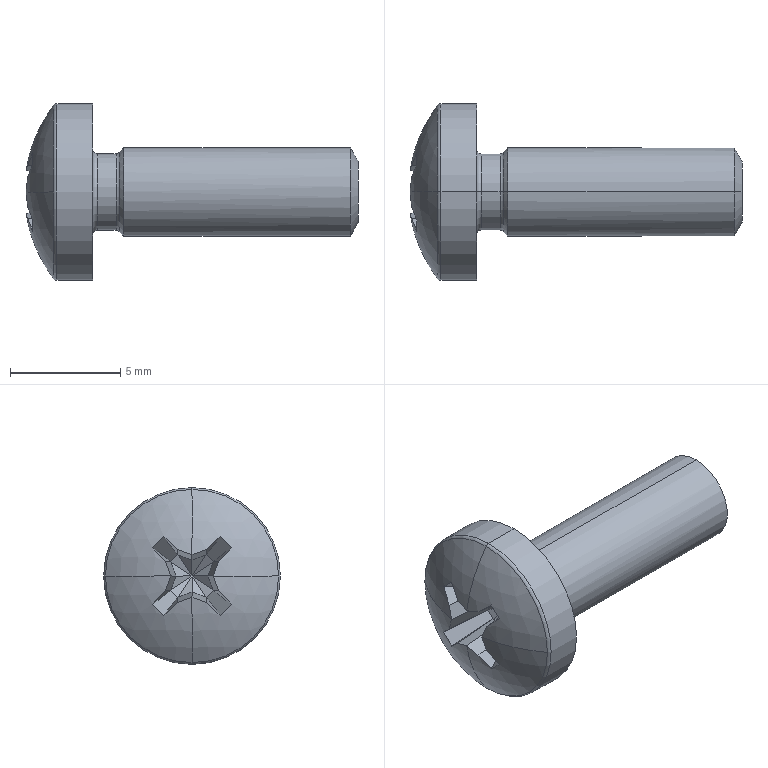Part | STEP file | 103000010384_M4×12 | 1 solid | 54 faces | box 15.027 x 8 x 8 mm | volume 256.338 mm3 | plane 34 | cylinder 6 | torus 6 | cone 4 | sphere 4 | commonest cylinder face diameters 3.464 x2 4 x2 8 x2
STEP:
#1=CARTESIAN_POINT('',(15.1,0.,1.394));
#2=VERTEX_POINT('',#1);
#3=CARTESIAN_POINT('',(15.1,0.,-1.394));
#4=VERTEX_POINT('',#3);
#5=CARTESIAN_POINT('',(15.1,0.,0.));
#6=DIRECTION('',(-1.,0.,0.));
#7=AXIS2_PLACEMENT_3D('',#5,#6,$);
#8=CIRCLE('',#7,1.394);
#9=EDGE_CURVE('',#2,#4,#8,.T.);
#10=ORIENTED_EDGE('',*,*,#9,.T.);
#11=CARTESIAN_POINT('',(14.754,0.,-2.));
#12=VERTEX_POINT('',#11);
#13=CARTESIAN_POINT('',(-247950.901,0.,-434181.551));
#14=DIRECTION('',(-0.4959,0.,-0.8684));
#15=VECTOR('',#14,1.);
#16=LINE('',#13,#15);
#17=EDGE_CURVE('',#4,#12,#16,.T.);
#18=ORIENTED_EDGE('',*,*,#17,.T.);
#19=CARTESIAN_POINT('',(14.754,0.,2.));
#20=VERTEX_POINT('',#19);
#21=CARTESIAN_POINT('',(14.754,0.,0.));
#22=DIRECTION('',(-1.,0.,0.));
#23=AXIS2_PLACEMENT_3D('',#21,#22,$);
#24=CIRCLE('',#23,2.);
#25=EDGE_CURVE('',#20,#12,#24,.T.);
#26=ORIENTED_EDGE('',*,*,#25,.F.);
#27=CARTESIAN_POINT('',(-247950.901,0.,434181.551));
#28=DIRECTION('',(-0.4959,0.,0.8684));
#29=VECTOR('',#28,1.);
#30=LINE('',#27,#29);
#31=EDGE_CURVE('',#2,#20,#30,.T.);
#32=ORIENTED_EDGE('',*,*,#31,.F.);
#33=EDGE_LOOP('',(#10,#18,#26,#32));
#34=FACE_OUTER_BOUND('',#33,.T.);
#35=CARTESIAN_POINT('',(14.754,0.,0.));
#36=DIRECTION('',(-1.,0.,0.));
#37=DIRECTION('',(0.,0.,1.));
#38=AXIS2_PLACEMENT_3D('',#35,#36,#37);
#39=CONICAL_SURFACE('',#38,2.,1.052);
#40=ADVANCED_FACE('',(#34),#39,.T.);
#41=ORIENTED_EDGE('',*,*,#9,.F.);
#42=CARTESIAN_POINT('',(15.1,0.,0.));
#43=DIRECTION('',(-1.,0.,0.));
#44=AXIS2_PLACEMENT_3D('',#42,#43,$);
#45=CIRCLE('',#44,1.394);
#46=EDGE_CURVE('',#4,#2,#45,.T.);
#47=ORIENTED_EDGE('',*,*,#46,.F.);
#48=EDGE_LOOP('',(#41,#47));
#49=FACE_OUTER_BOUND('',#48,.T.);
#50=CARTESIAN_POINT('',(15.1,0.,0.));
#51=DIRECTION('',(-1.,0.,0.));
#52=DIRECTION('',(0.,0.,1.));
#53=AXIS2_PLACEMENT_3D('',#50,#51,#52);
#54=PLANE('',#53);
#55=ADVANCED_FACE('',(#49),#54,.F.);
#56=ORIENTED_EDGE('',*,*,#17,.F.);
#57=ORIENTED_EDGE('',*,*,#46,.T.);
#58=ORIENTED_EDGE('',*,*,#31,.T.);
#59=CARTESIAN_POINT('',(14.754,0.,0.));
#60=DIRECTION('',(-1.,0.,0.));
#61=AXIS2_PLACEMENT_3D('',#59,#60,$);
#62=CIRCLE('',#61,2.);
#63=EDGE_CURVE('',#12,#20,#62,.T.);
#64=ORIENTED_EDGE('',*,*,#63,.F.);
#65=EDGE_LOOP('',(#56,#57,#58,#64));
#66=FACE_OUTER_BOUND('',#65,.T.);
#67=CARTESIAN_POINT('',(14.754,0.,0.));
#68=DIRECTION('',(-1.,0.,0.));
#69=DIRECTION('',(0.,0.,-1.));
#70=AXIS2_PLACEMENT_3D('',#67,#68,#69);
#71=CONICAL_SURFACE('',#70,2.,1.052);
#72=ADVANCED_FACE('',(#66),#71,.T.);
#73=ORIENTED_EDGE('',*,*,#25,.T.);
#74=CARTESIAN_POINT('',(4.5,0.,-2.));
#75=VERTEX_POINT('',#74);
#76=CARTESIAN_POINT('',(-3.442,0.,-2.));
#77=DIRECTION('',(-1.,0.,0.));
#78=VECTOR('',#77,1.);
#79=LINE('',#76,#78);
#80=EDGE_CURVE('',#12,#75,#79,.T.);
#81=ORIENTED_EDGE('',*,*,#80,.T.);
#82=CARTESIAN_POINT('',(4.5,0.,2.));
#83=VERTEX_POINT('',#82);
#84=CARTESIAN_POINT('',(4.5,0.,2.));
#85=CARTESIAN_POINT('',(4.5,0.6283,2.));
#86=CARTESIAN_POINT('',(4.5,1.257,1.753));
#87=CARTESIAN_POINT('',(4.5,1.753,1.257));
#88=CARTESIAN_POINT('',(4.5,2.247,0.));
#89=CARTESIAN_POINT('',(4.5,1.753,-1.257));
#90=CARTESIAN_POINT('',(4.5,1.257,-1.753));
#91=CARTESIAN_POINT('',(4.5,0.6283,-2.));
#92=CARTESIAN_POINT('',(4.5,0.,-2.));
#93=B_SPLINE_CURVE_WITH_KNOTS('',5,(#84,#85,#86,#87,#88,#89,#90,#91,#92),.UNSPECIFIED.,.F.,.U.,(6,3,6),(-3.142,0.,3.142),.UNSPECIFIED.);
#94=EDGE_CURVE('',#83,#75,#93,.T.);
#95=ORIENTED_EDGE('',*,*,#94,.F.);
#96=CARTESIAN_POINT('',(-3.442,0.,2.));
#97=DIRECTION('',(-1.,0.,0.));
#98=VECTOR('',#97,1.);
#99=LINE('',#96,#98);
#100=EDGE_CURVE('',#20,#83,#99,.T.);
#101=ORIENTED_EDGE('',*,*,#100,.F.);
#102=EDGE_LOOP('',(#73,#81,#95,#101));
#103=FACE_OUTER_BOUND('',#102,.T.);
#104=CARTESIAN_POINT('',(-3.442,0.,0.));
#105=DIRECTION('',(-1.,0.,0.));
#106=DIRECTION('',(0.,0.,1.));
#107=AXIS2_PLACEMENT_3D('',#104,#105,#106);
#108=CYLINDRICAL_SURFACE('',#107,2.);
#109=ADVANCED_FACE('',(#103),#108,.T.);
#110=ORIENTED_EDGE('',*,*,#80,.F.);
#111=ORIENTED_EDGE('',*,*,#63,.T.);
#112=ORIENTED_EDGE('',*,*,#100,.T.);
#113=CARTESIAN_POINT('',(4.5,0.,-2.));
#114=CARTESIAN_POINT('',(4.5,-0.6283,-2.));
#115=CARTESIAN_POINT('',(4.5,-1.257,-1.753));
#116=CARTESIAN_POINT('',(4.5,-1.753,-1.257));
#117=CARTESIAN_POINT('',(4.5,-2.247,0.));
#118=CARTESIAN_POINT('',(4.5,-1.753,1.257));
#119=CARTESIAN_POINT('',(4.5,-1.257,1.753));
#120=CARTESIAN_POINT('',(4.5,-0.6283,2.));
#121=CARTESIAN_POINT('',(4.5,0.,2.));
#122=B_SPLINE_CURVE_WITH_KNOTS('',5,(#113,#114,#115,#116,#117,#118,#119,#120,#121),.UNSPECIFIED.,.F.,.U.,(6,3,6),(-3.142,0.,3.142),.UNSPECIFIED.);
#123=EDGE_CURVE('',#75,#83,#122,.T.);
#124=ORIENTED_EDGE('',*,*,#123,.F.);
#125=EDGE_LOOP('',(#110,#111,#112,#124));
#126=FACE_OUTER_BOUND('',#125,.T.);
#127=CARTESIAN_POINT('',(-3.442,0.,0.));
#128=DIRECTION('',(-1.,0.,0.));
#129=DIRECTION('',(0.,0.,-1.));
#130=AXIS2_PLACEMENT_3D('',#127,#128,#129);
#131=CYLINDRICAL_SURFACE('',#130,2.);
#132=ADVANCED_FACE('',(#126),#131,.T.);
#133=CARTESIAN_POINT('',(4.291,0.,-1.791));
#134=VERTEX_POINT('',#133);
#135=CARTESIAN_POINT('',(4.291,0.,1.791));
#136=VERTEX_POINT('',#135);
#137=CARTESIAN_POINT('',(4.291,0.,0.));
#138=DIRECTION('',(1.,0.,0.));
#139=AXIS2_PLACEMENT_3D('',#137,#138,$);
#140=CIRCLE('',#139,1.791);
#141=EDGE_CURVE('',#134,#136,#140,.T.);
#142=ORIENTED_EDGE('',*,*,#141,.T.);
#143=CARTESIAN_POINT('',(353556.891,0.,353554.391));
#144=DIRECTION('',(0.7071,0.,0.7071));
#145=VECTOR('',#144,1.);
#146=LINE('',#143,#145);
#147=EDGE_CURVE('',#136,#83,#146,.T.);
#148=ORIENTED_EDGE('',*,*,#147,.T.);
#149=ORIENTED_EDGE('',*,*,#94,.T.);
#150=CARTESIAN_POINT('',(353556.891,0.,-353554.391));
#151=DIRECTION('',(0.7071,0.,-0.7071));
#152=VECTOR('',#151,1.);
#153=LINE('',#150,#152);
#154=EDGE_CURVE('',#134,#75,#153,.T.);
#155=ORIENTED_EDGE('',*,*,#154,.F.);
#156=EDGE_LOOP('',(#142,#148,#149,#155));
#157=FACE_OUTER_BOUND('',#156,.T.);
#158=CARTESIAN_POINT('',(4.5,0.,0.));
#159=DIRECTION('',(1.,0.,0.));
#160=DIRECTION('',(0.,0.,-1.));
#161=AXIS2_PLACEMENT_3D('',#158,#159,#160);
#162=CONICAL_SURFACE('',#161,2.,0.7854);
#163=ADVANCED_FACE('',(#157),#162,.T.);
#164=ORIENTED_EDGE('',*,*,#147,.F.);
#165=CARTESIAN_POINT('',(4.291,0.,0.));
#166=DIRECTION('',(1.,0.,0.));
#167=AXIS2_PLACEMENT_3D('',#165,#166,$);
#168=CIRCLE('',#167,1.791);
#169=EDGE_CURVE('',#136,#134,#168,.T.);
#170=ORIENTED_EDGE('',*,*,#169,.T.);
#171=ORIENTED_EDGE('',*,*,#154,.T.);
#172=ORIENTED_EDGE('',*,*,#123,.T.);
#173=EDGE_LOOP('',(#164,#170,#171,#172));
#174=FACE_OUTER_BOUND('',#173,.T.);
#175=CARTESIAN_POINT('',(4.5,0.,0.));
#176=DIRECTION('',(1.,0.,0.));
#177=DIRECTION('',(0.,0.,1.));
#178=AXIS2_PLACEMENT_3D('',#175,#176,#177);
#179=CONICAL_SURFACE('',#178,2.,0.7854);
#180=ADVANCED_FACE('',(#174),#179,.T.);
#181=CARTESIAN_POINT('',(4.149,0.,-1.732));
#182=VERTEX_POINT('',#181);
#183=CARTESIAN_POINT('',(4.149,0.,-1.932));
#184=DIRECTION('',(0.,1.,0.));
#185=AXIS2_PLACEMENT_3D('',#183,#184,$);
#186=CIRCLE('',#185,0.2);
#187=EDGE_CURVE('',#182,#134,#186,.T.);
#188=ORIENTED_EDGE('',*,*,#187,.F.);
#189=CARTESIAN_POINT('',(4.149,0.,1.732));
#190=VERTEX_POINT('',#189);
#191=CARTESIAN_POINT('',(4.149,0.,0.));
#192=DIRECTION('',(-1.,0.,0.));
#193=AXIS2_PLACEMENT_3D('',#191,#192,$);
#194=CIRCLE('',#193,1.732);
#195=EDGE_CURVE('',#190,#182,#194,.T.);
#196=ORIENTED_EDGE('',*,*,#195,.F.);
#197=CARTESIAN_POINT('',(4.149,0.,1.932));
#198=DIRECTION('',(0.,-1.,0.));
#199=AXIS2_PLACEMENT_3D('',#197,#198,$);
#200=CIRCLE('',#199,0.2);
#201=EDGE_CURVE('',#190,#136,#200,.T.);
#202=ORIENTED_EDGE('',*,*,#201,.T.);
#203=ORIENTED_EDGE('',*,*,#141,.F.);
#204=EDGE_LOOP('',(#188,#196,#202,#203));
#205=FACE_OUTER_BOUND('',#204,.T.);
#206=CARTESIAN_POINT('',(4.149,0.,0.));
#207=DIRECTION('',(-1.,0.,0.));
#208=DIRECTION('',(0.,0.,1.));
#209=AXIS2_PLACEMENT_3D('',#206,#207,#208);
#210=TOROIDAL_SURFACE('',#209,1.932,0.2);
#211=ADVANCED_FACE('',(#205),#210,.F.);
#212=CARTESIAN_POINT('',(4.149,0.,0.));
#213=DIRECTION('',(-1.,0.,0.));
#214=AXIS2_PLACEMENT_3D('',#212,#213,$);
#215=CIRCLE('',#214,1.732);
#216=EDGE_CURVE('',#182,#190,#215,.T.);
#217=ORIENTED_EDGE('',*,*,#216,.F.);
#218=ORIENTED_EDGE('',*,*,#187,.T.);
#219=ORIENTED_EDGE('',*,*,#169,.F.);
#220=ORIENTED_EDGE('',*,*,#201,.F.);
#221=EDGE_LOOP('',(#217,#218,#219,#220));
#222=FACE_OUTER_BOUND('',#221,.T.);
#223=CARTESIAN_POINT('',(4.149,0.,0.));
#224=DIRECTION('',(-1.,0.,0.));
#225=DIRECTION('',(0.,0.,-1.));
#226=AXIS2_PLACEMENT_3D('',#223,#224,#225);
#227=TOROIDAL_SURFACE('',#226,1.932,0.2);
#228=ADVANCED_FACE('',(#222),#227,.F.);
#229=ORIENTED_EDGE('',*,*,#195,.T.);
#230=CARTESIAN_POINT('',(3.3,0.,-1.732));
#231=VERTEX_POINT('',#230);
#232=CARTESIAN_POINT('',(-3.442,0.,-1.732));
#233=DIRECTION('',(-1.,0.,0.));
#234=VECTOR('',#233,1.);
#235=LINE('',#232,#234);
#236=EDGE_CURVE('',#182,#231,#235,.T.);
#237=ORIENTED_EDGE('',*,*,#236,.T.);
#238=CARTESIAN_POINT('',(3.3,0.,1.732));
#239=VERTEX_POINT('',#238);
#240=CARTESIAN_POINT('',(3.3,0.,0.));
#241=DIRECTION('',(-1.,0.,0.));
#242=AXIS2_PLACEMENT_3D('',#240,#241,$);
#243=CIRCLE('',#242,1.732);
#244=EDGE_CURVE('',#231,#239,#243,.F.);
#245=ORIENTED_EDGE('',*,*,#244,.T.);
#246=CARTESIAN_POINT('',(-3.442,0.,1.732));
#247=DIRECTION('',(-1.,0.,0.));
#248=VECTOR('',#247,1.);
#249=LINE('',#246,#248);
#250=EDGE_CURVE('',#190,#239,#249,.T.);
#251=ORIENTED_EDGE('',*,*,#250,.F.);
#252=EDGE_LOOP('',(#229,#237,#245,#251));
#253=FACE_OUTER_BOUND('',#252,.T.);
#254=CARTESIAN_POINT('',(-3.442,0.,0.));
#255=DIRECTION('',(-1.,0.,0.));
#256=DIRECTION('',(0.,0.,1.));
#257=AXIS2_PLACEMENT_3D('',#254,#255,#256);
#258=CYLINDRICAL_SURFACE('',#257,1.732);
#259=ADVANCED_FACE('',(#253),#258,.T.);
#260=ORIENTED_EDGE('',*,*,#236,.F.);
#261=ORIENTED_EDGE('',*,*,#216,.T.);
#262=ORIENTED_EDGE('',*,*,#250,.T.);
#263=CARTESIAN_POINT('',(3.3,0.,0.));
#264=DIRECTION('',(-1.,0.,0.));
#265=AXIS2_PLACEMENT_3D('',#263,#264,$);
#266=CIRCLE('',#265,1.732);
#267=EDGE_CURVE('',#239,#231,#266,.F.);
#268=ORIENTED_EDGE('',*,*,#267,.T.);
#269=EDGE_LOOP('',(#260,#261,#262,#268));
#270=FACE_OUTER_BOUND('',#269,.T.);
#271=CARTESIAN_POINT('',(-3.442,0.,0.));
#272=DIRECTION('',(-1.,0.,0.));
#273=DIRECTION('',(0.,0.,-1.));
#274=AXIS2_PLACEMENT_3D('',#271,#272,#273);
#275=CYLINDRICAL_SURFACE('',#274,1.732);
#276=ADVANCED_FACE('',(#270),#275,.T.);
#277=CARTESIAN_POINT('',(3.1,0.,-1.932));
#278=VERTEX_POINT('',#277);
#279=CARTESIAN_POINT('',(3.3,0.,-1.932));
#280=DIRECTION('',(0.,1.,0.));
#281=AXIS2_PLACEMENT_3D('',#279,#280,$);
#282=CIRCLE('',#281,0.2);
#283=EDGE_CURVE('',#278,#231,#282,.T.);
#284=ORIENTED_EDGE('',*,*,#283,.F.);
#285=CARTESIAN_POINT('',(3.1,0.,1.932));
#286=VERTEX_POINT('',#285);
#287=CARTESIAN_POINT('',(3.1,0.,0.));
#288=DIRECTION('',(-1.,0.,0.));
#289=AXIS2_PLACEMENT_3D('',#287,#288,$);
#290=CIRCLE('',#289,1.932);
#291=EDGE_CURVE('',#286,#278,#290,.T.);
#292=ORIENTED_EDGE('',*,*,#291,.F.);
#293=CARTESIAN_POINT('',(3.3,0.,1.932));
#294=DIRECTION('',(0.,-1.,0.));
#295=AXIS2_PLACEMENT_3D('',#293,#294,$);
#296=CIRCLE('',#295,0.2);
#297=EDGE_CURVE('',#286,#239,#296,.T.);
#298=ORIENTED_EDGE('',*,*,#297,.T.);
#299=ORIENTED_EDGE('',*,*,#244,.F.);
#300=EDGE_LOOP('',(#284,#292,#298,#299));
#301=FACE_OUTER_BOUND('',#300,.T.);
#302=CARTESIAN_POINT('',(3.3,0.,0.));
#303=DIRECTION('',(-1.,0.,0.));
#304=DIRECTION('',(0.,0.,1.));
#305=AXIS2_PLACEMENT_3D('',#302,#303,#304);
#306=TOROIDAL_SURFACE('',#305,1.932,0.2);
#307=ADVANCED_FACE('',(#301),#306,.F.);
#308=CARTESIAN_POINT('',(3.1,0.,0.));
#309=DIRECTION('',(-1.,0.,0.));
#310=AXIS2_PLACEMENT_3D('',#308,#309,$);
#311=CIRCLE('',#310,1.932);
#312=EDGE_CURVE('',#278,#286,#311,.T.);
#313=ORIENTED_EDGE('',*,*,#312,.F.);
#314=ORIENTED_EDGE('',*,*,#283,.T.);
#315=ORIENTED_EDGE('',*,*,#267,.F.);
#316=ORIENTED_EDGE('',*,*,#297,.F.);
#317=EDGE_LOOP('',(#313,#314,#315,#316));
#318=FACE_OUTER_BOUND('',#317,.T.);
#319=CARTESIAN_POINT('',(3.3,0.,0.));
#320=DIRECTION('',(-1.,0.,0.));
#321=DIRECTION('',(0.,0.,-1.));
#322=AXIS2_PLACEMENT_3D('',#319,#320,#321);
#323=TOROIDAL_SURFACE('',#322,1.932,0.2);
#324=ADVANCED_FACE('',(#318),#323,.F.);
#325=CARTESIAN_POINT('',(3.1,0.,4.));
#326=VERTEX_POINT('',#325);
#327=CARTESIAN_POINT('',(3.1,0.,-4.));
#328=VERTEX_POINT('',#327);
#329=CARTESIAN_POINT('',(3.1,0.,0.));
#330=DIRECTION('',(-1.,0.,0.));
#331=AXIS2_PLACEMENT_3D('',#329,#330,$);
#332=CIRCLE('',#331,4.);
#333=EDGE_CURVE('',#326,#328,#332,.T.);
#334=ORIENTED_EDGE('',*,*,#333,.F.);
#335=CARTESIAN_POINT('',(3.1,0.,0.));
#336=DIRECTION('',(-1.,0.,0.));
#337=AXIS2_PLACEMENT_3D('',#335,#336,$);
#338=CIRCLE('',#337,4.);
#339=EDGE_CURVE('',#328,#326,#338,.T.);
#340=ORIENTED_EDGE('',*,*,#339,.F.);
#341=EDGE_LOOP('',(#334,#340));
#342=FACE_OUTER_BOUND('',#341,.T.);
#343=ORIENTED_EDGE('',*,*,#291,.T.);
#344=ORIENTED_EDGE('',*,*,#312,.T.);
#345=EDGE_LOOP('',(#343,#344));
#346=FACE_BOUND('',#345,.T.);
#347=CARTESIAN_POINT('',(3.1,4.,0.));
#348=DIRECTION('',(-1.,0.,0.));
#349=DIRECTION('',(0.,0.,1.));
#350=AXIS2_PLACEMENT_3D('',#347,#348,#349);
#351=PLANE('',#350);
#352=ADVANCED_FACE('',(#342,#346),#351,.F.);
#353=ORIENTED_EDGE('',*,*,#333,.T.);
#354=CARTESIAN_POINT('',(1.475,0.,-4.));
#355=VERTEX_POINT('',#354);
#356=CARTESIAN_POINT('',(-3.442,0.,-4.));
#357=DIRECTION('',(-1.,0.,0.));
#358=VECTOR('',#357,1.);
#359=LINE('',#356,#358);
#360=EDGE_CURVE('',#328,#355,#359,.T.);
#361=ORIENTED_EDGE('',*,*,#360,.T.);
#362=CARTESIAN_POINT('',(1.475,0.,4.));
#363=VERTEX_POINT('',#362);
#364=CARTESIAN_POINT('',(1.475,0.,0.));
#365=DIRECTION('',(-1.,0.,0.));
#366=AXIS2_PLACEMENT_3D('',#364,#365,$);
#367=CIRCLE('',#366,4.);
#368=EDGE_CURVE('',#355,#363,#367,.F.);
#369=ORIENTED_EDGE('',*,*,#368,.T.);
#370=CARTESIAN_POINT('',(-3.442,0.,4.));
#371=DIRECTION('',(-1.,0.,0.));
#372=VECTOR('',#371,1.);
#373=LINE('',#370,#372);
#374=EDGE_CURVE('',#326,#363,#373,.T.);
#375=ORIENTED_EDGE('',*,*,#374,.F.);
#376=EDGE_LOOP('',(#353,#361,#369,#375));
#377=FACE_OUTER_BOUND('',#376,.T.);
#378=CARTESIAN_POINT('',(-3.442,0.,0.));
#379=DIRECTION('',(-1.,0.,0.));
#380=DIRECTION('',(0.,0.,1.));
#381=AXIS2_PLACEMENT_3D('',#378,#379,#380);
#382=CYLINDRICAL_SURFACE('',#381,4.);
#383=ADVANCED_FACE('',(#377),#382,.T.);
#384=ORIENTED_EDGE('',*,*,#360,.F.);
#385=ORIENTED_EDGE('',*,*,#339,.T.);
#386=ORIENTED_EDGE('',*,*,#374,.T.);
#387=CARTESIAN_POINT('',(1.475,0.,0.));
#388=DIRECTION('',(-1.,0.,0.));
#389=AXIS2_PLACEMENT_3D('',#387,#388,$);
#390=CIRCLE('',#389,4.);
#391=EDGE_CURVE('',#363,#355,#390,.F.);
#392=ORIENTED_EDGE('',*,*,#391,.T.);
#393=EDGE_LOOP('',(#384,#385,#386,#392));
#394=FACE_OUTER_BOUND('',#393,.T.);
#395=CARTESIAN_POINT('',(-3.442,0.,0.));
#396=DIRECTION('',(-1.,0.,0.));
#397=DIRECTION('',(0.,0.,-1.));
#398=AXIS2_PLACEMENT_3D('',#395,#396,#397);
#399=CYLINDRICAL_SURFACE('',#398,4.);
#400=ADVANCED_FACE('',(#394),#399,.T.);
#401=CARTESIAN_POINT('',(1.316,0.,3.921));
#402=VERTEX_POINT('',#401);
#403=CARTESIAN_POINT('',(1.316,3.921,0.));
#404=VERTEX_POINT('',#403);
#405=CARTESIAN_POINT('',(1.316,0.,0.));
#406=DIRECTION('',(1.,0.,0.));
#407=AXIS2_PLACEMENT_3D('',#405,#406,$);
#408=CIRCLE('',#407,3.921);
#409=EDGE_CURVE('',#402,#404,#408,.F.);
#410=ORIENTED_EDGE('',*,*,#409,.F.);
#411=CARTESIAN_POINT('',(1.475,0.,3.8));
#412=DIRECTION('',(0.,1.,0.));
#413=AXIS2_PLACEMENT_3D('',#411,#412,$);
#414=CIRCLE('',#413,0.2);
#415=EDGE_CURVE('',#402,#363,#414,.T.);
#416=ORIENTED_EDGE('',*,*,#415,.T.);
#417=ORIENTED_EDGE('',*,*,#368,.F.);
#418=CARTESIAN_POINT('',(1.316,0.,-3.921));
#419=VERTEX_POINT('',#418);
#420=CARTESIAN_POINT('',(1.475,0.,-3.8));
#421=DIRECTION('',(0.,-1.,0.));
#422=AXIS2_PLACEMENT_3D('',#420,#421,$);
#423=CIRCLE('',#422,0.2);
#424=EDGE_CURVE('',#419,#355,#423,.T.);
#425=ORIENTED_EDGE('',*,*,#424,.F.);
#426=CARTESIAN_POINT('',(1.316,0.,0.));
#427=DIRECTION('',(1.,0.,0.));
#428=AXIS2_PLACEMENT_3D('',#426,#427,$);
#429=CIRCLE('',#428,3.921);
#430=EDGE_CURVE('',#404,#419,#429,.F.);
#431=ORIENTED_EDGE('',*,*,#430,.F.);
#432=EDGE_LOOP('',(#410,#416,#417,#425,#431));
#433=FACE_OUTER_BOUND('',#432,.T.);
#434=CARTESIAN_POINT('',(1.475,0.,0.));
#435=DIRECTION('',(1.,0.,0.));
#436=DIRECTION('',(0.,0.,-1.));
#437=AXIS2_PLACEMENT_3D('',#434,#435,#436);
#438=TOROIDAL_SURFACE('',#437,3.8,0.2);
#439=ADVANCED_FACE('',(#433),#438,.T.);
#440=ORIENTED_EDGE('',*,*,#415,.F.);
#441=CARTESIAN_POINT('',(1.316,-3.921,0.));
#442=VERTEX_POINT('',#441);
#443=CARTESIAN_POINT('',(1.316,0.,0.));
#444=DIRECTION('',(1.,0.,0.));
#445=AXIS2_PLACEMENT_3D('',#443,#444,$);
#446=CIRCLE('',#445,3.921);
#447=EDGE_CURVE('',#442,#402,#446,.F.);
#448=ORIENTED_EDGE('',*,*,#447,.F.);
#449=CARTESIAN_POINT('',(1.316,0.,0.));
#450=DIRECTION('',(1.,0.,0.));
#451=AXIS2_PLACEMENT_3D('',#449,#450,$);
#452=CIRCLE('',#451,3.921);
#453=EDGE_CURVE('',#419,#442,#452,.F.);
#454=ORIENTED_EDGE('',*,*,#453,.F.);
#455=ORIENTED_EDGE('',*,*,#424,.T.);
#456=ORIENTED_EDGE('',*,*,#391,.F.);
#457=EDGE_LOOP('',(#440,#448,#454,#455,#456));
#458=FACE_OUTER_BOUND('',#457,.T.);
#459=CARTESIAN_POINT('',(1.475,0.,0.));
#460=DIRECTION('',(1.,0.,0.));
#461=DIRECTION('',(0.,0.,1.));
#462=AXIS2_PLACEMENT_3D('',#459,#460,#461);
#463=TOROIDAL_SURFACE('',#462,3.8,0.2);
#464=ADVANCED_FACE('',(#458),#463,.T.);
#465=CARTESIAN_POINT('',(0.07269,0.,0.9693));
#466=VERTEX_POINT('',#465);
#467=CARTESIAN_POINT('',(6.5,0.,0.));
#468=DIRECTION('',(0.,-1.,0.));
#469=AXIS2_PLACEMENT_3D('',#467,#468,$);
#470=CIRCLE('',#469,6.5);
#471=EDGE_CURVE('',#402,#466,#470,.T.);
#472=ORIENTED_EDGE('',*,*,#471,.F.);
#473=ORIENTED_EDGE('',*,*,#409,.T.);
#474=CARTESIAN_POINT('',(0.07269,0.9693,0.));
#475=VERTEX_POINT('',#474);
#476=CARTESIAN_POINT('',(6.5,0.,0.));
#477=DIRECTION('',(0.,0.,-1.));
#478=AXIS2_PLACEMENT_3D('',#476,#477,$);
#479=CIRCLE('',#478,6.5);
#480=EDGE_CURVE('',#404,#475,#479,.F.);
#481=ORIENTED_EDGE('',*,*,#480,.T.);
#482=CARTESIAN_POINT('',(0.1444,1.198,0.6483));
#483=VERTEX_POINT('',#482);
#484=CARTESIAN_POINT('',(0.07269,0.9693,0.));
#485=CARTESIAN_POINT('',(0.0844,1.047,0.2167));
#486=CARTESIAN_POINT('',(0.1083,1.123,0.4333));
#487=CARTESIAN_POINT('',(0.1444,1.198,0.6483));
#488=B_SPLINE_CURVE_WITH_KNOTS('',3,(#484,#485,#486,#487),.UNSPECIFIED.,.F.,.U.,(4,4),(0.,0.9781),.UNSPECIFIED.);
#489=EDGE_CURVE('',#475,#483,#488,.T.);
#490=ORIENTED_EDGE('',*,*,#489,.T.);
#491=CARTESIAN_POINT('',(0.3775,1.775,1.27));
#492=VERTEX_POINT('',#491);
#493=CARTESIAN_POINT('',(0.1444,1.198,0.6483));
#494=CARTESIAN_POINT('',(0.2029,1.395,0.8585));
#495=CARTESIAN_POINT('',(0.281,1.588,1.066));
#496=CARTESIAN_POINT('',(0.3775,1.775,1.27));
#497=B_SPLINE_CURVE_WITH_KNOTS('',3,(#493,#494,#495,#496),.UNSPECIFIED.,.F.,.U.,(4,4),(0.,1.249),.UNSPECIFIED.);
#498=EDGE_CURVE('',#483,#492,#497,.T.);
#499=ORIENTED_EDGE('',*,*,#498,.T.);
#500=CARTESIAN_POINT('',(0.3775,1.27,1.775));
#501=VERTEX_POINT('',#500);
#502=CARTESIAN_POINT('',(0.3775,1.27,1.775));
#503=CARTESIAN_POINT('',(0.3657,1.442,1.612));
#504=CARTESIAN_POINT('',(0.3656,1.611,1.443));
#505=CARTESIAN_POINT('',(0.3775,1.775,1.27));
#506=B_SPLINE_CURVE_WITH_KNOTS('',3,(#502,#503,#504,#505),.UNSPECIFIED.,.F.,.U.,(4,4),(0.,1.017),.UNSPECIFIED.);
#507=EDGE_CURVE('',#501,#492,#506,.T.);
#508=ORIENTED_EDGE('',*,*,#507,.F.);
#509=CARTESIAN_POINT('',(0.1444,0.6483,1.198));
#510=VERTEX_POINT('',#509);
#511=CARTESIAN_POINT('',(0.3775,1.27,1.775));
#512=CARTESIAN_POINT('',(0.2811,1.067,1.588));
#513=CARTESIAN_POINT('',(0.203,0.8587,1.395));
#514=CARTESIAN_POINT('',(0.1444,0.6483,1.198));
#515=B_SPLINE_CURVE_WITH_KNOTS('',3,(#511,#512,#513,#514),.UNSPECIFIED.,.F.,.U.,(4,4),(0.,1.255),.UNSPECIFIED.);
#516=EDGE_CURVE('',#501,#510,#515,.T.);
#517=ORIENTED_EDGE('',*,*,#516,.T.);
#518=CARTESIAN_POINT('',(0.1444,0.6483,1.198));
#519=CARTESIAN_POINT('',(0.1084,0.4335,1.124));
#520=CARTESIAN_POINT('',(0.08442,0.217,1.047));
#521=CARTESIAN_POINT('',(0.07269,0.,0.9693));
#522=B_SPLINE_CURVE_WITH_KNOTS('',3,(#518,#519,#520,#521),.UNSPECIFIED.,.F.,.U.,(4,4),(0.,0.9842),.UNSPECIFIED.);
#523=EDGE_CURVE('',#510,#466,#522,.T.);
#524=ORIENTED_EDGE('',*,*,#523,.T.);
#525=EDGE_LOOP('',(#472,#473,#481,#490,#499,#508,#517,#524));
#526=FACE_OUTER_BOUND('',#525,.T.);
#527=CARTESIAN_POINT('',(6.5,0.,0.));
#528=DIRECTION('',(0.,0.,-1.));
#529=DIRECTION('',(-1.,0.,0.));
#530=AXIS2_PLACEMENT_3D('',#527,#528,#529);
#531=SPHERICAL_SURFACE('',#530,6.5);
#532=ADVANCED_FACE('',(#526),#531,.T.);
#533=CARTESIAN_POINT('',(0.07269,0.,-0.9693));
#534=VERTEX_POINT('',#533);
#535=CARTESIAN_POINT('',(6.5,0.,0.));
#536=DIRECTION('',(0.,-1.,0.));
#537=AXIS2_PLACEMENT_3D('',#535,#536,$);
#538=CIRCLE('',#537,6.5);
#539=EDGE_CURVE('',#534,#419,#538,.T.);
#540=ORIENTED_EDGE('',*,*,#539,.F.);
#541=CARTESIAN_POINT('',(0.1444,0.6483,-1.198));
#542=VERTEX_POINT('',#541);
#543=CARTESIAN_POINT('',(0.07269,0.,-0.9693));
#544=CARTESIAN_POINT('',(0.08442,0.217,-1.047));
#545=CARTESIAN_POINT('',(0.1084,0.4335,-1.124));
#546=CARTESIAN_POINT('',(0.1444,0.6483,-1.198));
#547=B_SPLINE_CURVE_WITH_KNOTS('',3,(#543,#544,#545,#546),.UNSPECIFIED.,.F.,.U.,(4,4),(0.,0.9842),.UNSPECIFIED.);
#548=EDGE_CURVE('',#534,#542,#547,.T.);
#549=ORIENTED_EDGE('',*,*,#548,.T.);
#550=CARTESIAN_POINT('',(0.3775,1.27,-1.775));
#551=VERTEX_POINT('',#550);
#552=CARTESIAN_POINT('',(0.1444,0.6483,-1.198));
#553=CARTESIAN_POINT('',(0.203,0.8587,-1.395));
#554=CARTESIAN_POINT('',(0.2811,1.067,-1.588));
#555=CARTESIAN_POINT('',(0.3775,1.27,-1.775));
#556=B_SPLINE_CURVE_WITH_KNOTS('',3,(#552,#553,#554,#555),.UNSPECIFIED.,.F.,.U.,(4,4),(0.,1.255),.UNSPECIFIED.);
#557=EDGE_CURVE('',#542,#551,#556,.T.);
#558=ORIENTED_EDGE('',*,*,#557,.T.);
#559=CARTESIAN_POINT('',(0.3775,1.775,-1.27));
#560=VERTEX_POINT('',#559);
#561=CARTESIAN_POINT('',(0.3775,1.775,-1.27));
#562=CARTESIAN_POINT('',(0.3656,1.611,-1.443));
#563=CARTESIAN_POINT('',(0.3657,1.442,-1.612));
#564=CARTESIAN_POINT('',(0.3775,1.27,-1.775));
#565=B_SPLINE_CURVE_WITH_KNOTS('',3,(#561,#562,#563,#564),.UNSPECIFIED.,.F.,.U.,(4,4),(0.,1.017),.UNSPECIFIED.);
#566=EDGE_CURVE('',#560,#551,#565,.T.);
#567=ORIENTED_EDGE('',*,*,#566,.F.);
#568=CARTESIAN_POINT('',(0.1444,1.198,-0.6483));
#569=VERTEX_POINT('',#568);
#570=CARTESIAN_POINT('',(0.3775,1.775,-1.27));
#571=CARTESIAN_POINT('',(0.281,1.588,-1.066));
#572=CARTESIAN_POINT('',(0.2029,1.395,-0.8585));
#573=CARTESIAN_POINT('',(0.1444,1.198,-0.6483));
#574=B_SPLINE_CURVE_WITH_KNOTS('',3,(#570,#571,#572,#573),.UNSPECIFIED.,.F.,.U.,(4,4),(0.,1.249),.UNSPECIFIED.);
#575=EDGE_CURVE('',#560,#569,#574,.T.);
#576=ORIENTED_EDGE('',*,*,#575,.T.);
#577=CARTESIAN_POINT('',(0.1444,1.198,-0.6483));
#578=CARTESIAN_POINT('',(0.1083,1.123,-0.4333));
#579=CARTESIAN_POINT('',(0.0844,1.047,-0.2167));
#580=CARTESIAN_POINT('',(0.07269,0.9693,0.));
#581=B_SPLINE_CURVE_WITH_KNOTS('',3,(#577,#578,#579,#580),.UNSPECIFIED.,.F.,.U.,(4,4),(0.,0.9781),.UNSPECIFIED.);
#582=EDGE_CURVE('',#569,#475,#581,.T.);
#583=ORIENTED_EDGE('',*,*,#582,.T.);
#584=ORIENTED_EDGE('',*,*,#480,.F.);
#585=ORIENTED_EDGE('',*,*,#430,.T.);
#586=EDGE_LOOP('',(#540,#549,#558,#567,#576,#583,#584,#585));
#587=FACE_OUTER_BOUND('',#586,.T.);
#588=CARTESIAN_POINT('',(6.5,0.,0.));
#589=DIRECTION('',(0.,0.,-1.));
#590=DIRECTION('',(-1.,0.,0.));
#591=AXIS2_PLACEMENT_3D('',#588,#589,#590);
#592=SPHERICAL_SURFACE('',#591,6.5);
#593=ADVANCED_FACE('',(#587),#592,.T.);
#594=ORIENTED_EDGE('',*,*,#471,.T.);
#595=CARTESIAN_POINT('',(0.1444,-0.6483,1.198));
#596=VERTEX_POINT('',#595);
#597=CARTESIAN_POINT('',(0.07269,0.,0.9693));
#598=CARTESIAN_POINT('',(0.08442,-0.217,1.047));
#599=CARTESIAN_POINT('',(0.1084,-0.4335,1.124));
#600=CARTESIAN_POINT('',(0.1444,-0.6483,1.198));
#601=B_SPLINE_CURVE_WITH_KNOTS('',3,(#597,#598,#599,#600),.UNSPECIFIED.,.F.,.U.,(4,4),(0.,0.9842),.UNSPECIFIED.);
#602=EDGE_CURVE('',#466,#596,#601,.T.);
#603=ORIENTED_EDGE('',*,*,#602,.T.);
#604=CARTESIAN_POINT('',(0.3775,-1.27,1.775));
#605=VERTEX_POINT('',#604);
#606=CARTESIAN_POINT('',(0.1444,-0.6483,1.198));
#607=CARTESIAN_POINT('',(0.203,-0.8587,1.395));
#608=CARTESIAN_POINT('',(0.2811,-1.067,1.588));
#609=CARTESIAN_POINT('',(0.3775,-1.27,1.775));
#610=B_SPLINE_CURVE_WITH_KNOTS('',3,(#606,#607,#608,#609),.UNSPECIFIED.,.F.,.U.,(4,4),(0.,1.255),.UNSPECIFIED.);
#611=EDGE_CURVE('',#596,#605,#610,.T.);
#612=ORIENTED_EDGE('',*,*,#611,.T.);
#613=CARTESIAN_POINT('',(0.3775,-1.775,1.27));
#614=VERTEX_POINT('',#613);
#615=CARTESIAN_POINT('',(0.3775,-1.775,1.27));
#616=CARTESIAN_POINT('',(0.3656,-1.611,1.443));
#617=CARTESIAN_POINT('',(0.3657,-1.442,1.612));
#618=CARTESIAN_POINT('',(0.3775,-1.27,1.775));
#619=B_SPLINE_CURVE_WITH_KNOTS('',3,(#615,#616,#617,#618),.UNSPECIFIED.,.F.,.U.,(4,4),(0.,1.017),.UNSPECIFIED.);
#620=EDGE_CURVE('',#614,#605,#619,.T.);
#621=ORIENTED_EDGE('',*,*,#620,.F.);
#622=CARTESIAN_POINT('',(0.1444,-1.198,0.6483));
#623=VERTEX_POINT('',#622);
#624=CARTESIAN_POINT('',(0.3775,-1.775,1.27));
#625=CARTESIAN_POINT('',(0.281,-1.588,1.066));
#626=CARTESIAN_POINT('',(0.2029,-1.395,0.8585));
#627=CARTESIAN_POINT('',(0.1444,-1.198,0.6483));
#628=B_SPLINE_CURVE_WITH_KNOTS('',3,(#624,#625,#626,#627),.UNSPECIFIED.,.F.,.U.,(4,4),(0.,1.249),.UNSPECIFIED.);
#629=EDGE_CURVE('',#614,#623,#628,.T.);
#630=ORIENTED_EDGE('',*,*,#629,.T.);
#631=CARTESIAN_POINT('',(0.07269,-0.9693,0.));
#632=VERTEX_POINT('',#631);
#633=CARTESIAN_POINT('',(0.1444,-1.198,0.6483));
#634=CARTESIAN_POINT('',(0.1083,-1.123,0.4333));
#635=CARTESIAN_POINT('',(0.0844,-1.047,0.2167));
#636=CARTESIAN_POINT('',(0.07269,-0.9693,0.));
#637=B_SPLINE_CURVE_WITH_KNOTS('',3,(#633,#634,#635,#636),.UNSPECIFIED.,.F.,.U.,(4,4),(0.,0.9781),.UNSPECIFIED.);
#638=EDGE_CURVE('',#623,#632,#637,.T.);
#639=ORIENTED_EDGE('',*,*,#638,.T.);
#640=CARTESIAN_POINT('',(6.5,0.,0.));
#641=DIRECTION('',(0.,0.,-1.));
#642=AXIS2_PLACEMENT_3D('',#640,#641,$);
#643=CIRCLE('',#642,6.5);
#644=EDGE_CURVE('',#442,#632,#643,.T.);
#645=ORIENTED_EDGE('',*,*,#644,.F.);
#646=ORIENTED_EDGE('',*,*,#447,.T.);
#647=EDGE_LOOP('',(#594,#603,#612,#621,#630,#639,#645,#646));
#648=FACE_OUTER_BOUND('',#647,.T.);
#649=CARTESIAN_POINT('',(6.5,0.,0.));
#650=DIRECTION('',(0.,0.,-1.));
#651=DIRECTION('',(0.,-1.,0.));
#652=AXIS2_PLACEMENT_3D('',#649,#650,#651);
#653=SPHERICAL_SURFACE('',#652,6.5);
#654=ADVANCED_FACE('',(#648),#653,.T.);
#655=ORIENTED_EDGE('',*,*,#539,.T.);
#656=ORIENTED_EDGE('',*,*,#453,.T.);
#657=ORIENTED_EDGE('',*,*,#644,.T.);
#658=CARTESIAN_POINT('',(0.1444,-1.198,-0.6483));
#659=VERTEX_POINT('',#658);
#660=CARTESIAN_POINT('',(0.07269,-0.9693,0.));
#661=CARTESIAN_POINT('',(0.0844,-1.047,-0.2167));
#662=CARTESIAN_POINT('',(0.1083,-1.123,-0.4333));
#663=CARTESIAN_POINT('',(0.1444,-1.198,-0.6483));
#664=B_SPLINE_CURVE_WITH_KNOTS('',3,(#660,#661,#662,#663),.UNSPECIFIED.,.F.,.U.,(4,4),(0.,0.9781),.UNSPECIFIED.);
#665=EDGE_CURVE('',#632,#659,#664,.T.);
#666=ORIENTED_EDGE('',*,*,#665,.T.);
#667=CARTESIAN_POINT('',(0.3775,-1.775,-1.27));
#668=VERTEX_POINT('',#667);
#669=CARTESIAN_POINT('',(0.1444,-1.198,-0.6483));
#670=CARTESIAN_POINT('',(0.2029,-1.395,-0.8585));
#671=CARTESIAN_POINT('',(0.281,-1.588,-1.066));
#672=CARTESIAN_POINT('',(0.3775,-1.775,-1.27));
#673=B_SPLINE_CURVE_WITH_KNOTS('',3,(#669,#670,#671,#672),.UNSPECIFIED.,.F.,.U.,(4,4),(0.,1.249),.UNSPECIFIED.);
#674=EDGE_CURVE('',#659,#668,#673,.T.);
#675=ORIENTED_EDGE('',*,*,#674,.T.);
#676=CARTESIAN_POINT('',(0.3775,-1.27,-1.775));
#677=VERTEX_POINT('',#676);
#678=CARTESIAN_POINT('',(0.3775,-1.27,-1.775));
#679=CARTESIAN_POINT('',(0.3657,-1.442,-1.612));
#680=CARTESIAN_POINT('',(0.3656,-1.611,-1.443));
#681=CARTESIAN_POINT('',(0.3775,-1.775,-1.27));
#682=B_SPLINE_CURVE_WITH_KNOTS('',3,(#678,#679,#680,#681),.UNSPECIFIED.,.F.,.U.,(4,4),(0.,1.017),.UNSPECIFIED.);
#683=EDGE_CURVE('',#677,#668,#682,.T.);
#684=ORIENTED_EDGE('',*,*,#683,.F.);
#685=CARTESIAN_POINT('',(0.1444,-0.6483,-1.198));
#686=VERTEX_POINT('',#685);
#687=CARTESIAN_POINT('',(0.3775,-1.27,-1.775));
#688=CARTESIAN_POINT('',(0.2811,-1.067,-1.588));
#689=CARTESIAN_POINT('',(0.203,-0.8587,-1.395));
#690=CARTESIAN_POINT('',(0.1444,-0.6483,-1.198));
#691=B_SPLINE_CURVE_WITH_KNOTS('',3,(#687,#688,#689,#690),.UNSPECIFIED.,.F.,.U.,(4,4),(0.,1.255),.UNSPECIFIED.);
#692=EDGE_CURVE('',#677,#686,#691,.T.);
#693=ORIENTED_EDGE('',*,*,#692,.T.);
#694=CARTESIAN_POINT('',(0.1444,-0.6483,-1.198));
#695=CARTESIAN_POINT('',(0.1084,-0.4335,-1.124));
#696=CARTESIAN_POINT('',(0.08442,-0.217,-1.047));
#697=CARTESIAN_POINT('',(0.07269,0.,-0.9693));
#698=B_SPLINE_CURVE_WITH_KNOTS('',3,(#694,#695,#696,#697),.UNSPECIFIED.,.F.,.U.,(4,4),(0.,0.9842),.UNSPECIFIED.);
#699=EDGE_CURVE('',#686,#534,#698,.T.);
#700=ORIENTED_EDGE('',*,*,#699,.T.);
#701=EDGE_LOOP('',(#655,#656,#657,#666,#675,#684,#693,#700));
#702=FACE_OUTER_BOUND('',#701,.T.);
#703=CARTESIAN_POINT('',(6.5,0.,0.));
#704=DIRECTION('',(0.,0.,-1.));
#705=DIRECTION('',(0.,-1.,0.));
#706=AXIS2_PLACEMENT_3D('',#703,#704,#705);
#707=SPHERICAL_SURFACE('',#706,6.5);
#708=ADVANCED_FACE('',(#702),#707,.T.);
#709=CARTESIAN_POINT('',(2.4,0.735,0.));
#710=VERTEX_POINT('',#709);
#711=CARTESIAN_POINT('',(1.236,0.8522,0.));
#712=DIRECTION('',(0.995,-0.1002,0.));
#713=VECTOR('',#712,1.);
#714=LINE('',#711,#713);
#715=EDGE_CURVE('',#475,#710,#714,.T.);
#716=ORIENTED_EDGE('',*,*,#715,.T.);
#717=CARTESIAN_POINT('',(2.4,0.971,0.6483));
#718=VERTEX_POINT('',#717);
#719=CARTESIAN_POINT('',(2.4,0.853,0.3242));
#720=DIRECTION('',(0.,0.342,0.9397));
#721=VECTOR('',#720,1.);
#722=LINE('',#719,#721);
#723=EDGE_CURVE('',#710,#718,#722,.T.);
#724=ORIENTED_EDGE('',*,*,#723,.T.);
#725=CARTESIAN_POINT('',(1.272,1.085,0.6483));
#726=DIRECTION('',(0.995,-0.1002,0.));
#727=VECTOR('',#726,1.);
#728=LINE('',#725,#727);
#729=EDGE_CURVE('',#483,#718,#728,.T.);
#730=ORIENTED_EDGE('',*,*,#729,.F.);
#731=ORIENTED_EDGE('',*,*,#489,.F.);
#732=EDGE_LOOP('',(#716,#724,#730,#731));
#733=FACE_OUTER_BOUND('',#732,.T.);
#734=CARTESIAN_POINT('',(0.,0.9767,0.));
#735=DIRECTION('',(0.0942,0.9355,-0.3405));
#736=DIRECTION('',(0.,0.342,0.9397));
#737=AXIS2_PLACEMENT_3D('',#734,#735,#736);
#738=PLANE('',#737);
#739=ADVANCED_FACE('',(#733),#738,.F.);
#740=ORIENTED_EDGE('',*,*,#729,.T.);
#741=CARTESIAN_POINT('',(1.389,1.373,0.9593));
#742=DIRECTION('',(0.8935,-0.3553,-0.2747));
#743=VECTOR('',#742,1.);
#744=LINE('',#741,#743);
#745=EDGE_CURVE('',#492,#718,#744,.T.);
#746=ORIENTED_EDGE('',*,*,#745,.F.);
#747=ORIENTED_EDGE('',*,*,#498,.F.);
#748=EDGE_LOOP('',(#740,#746,#747));
#749=FACE_OUTER_BOUND('',#748,.T.);
#750=CARTESIAN_POINT('',(0.,1.213,0.6483));
#751=DIRECTION('',(0.07224,0.7175,-0.6928));
#752=DIRECTION('',(0.,0.6947,0.7193));
#753=AXIS2_PLACEMENT_3D('',#750,#751,#752);
#754=PLANE('',#753);
#755=ADVANCED_FACE('',(#749),#754,.F.);
#756=ORIENTED_EDGE('',*,*,#507,.T.);
#757=ORIENTED_EDGE('',*,*,#745,.T.);
#758=CARTESIAN_POINT('',(2.4,0.6483,0.971));
#759=VERTEX_POINT('',#758);
#760=CARTESIAN_POINT('',(2.4,0.8096,0.8096));
#761=DIRECTION('',(0.,-0.7071,0.7071));
#762=VECTOR('',#761,1.);
#763=LINE('',#760,#762);
#764=EDGE_CURVE('',#718,#759,#763,.T.);
#765=ORIENTED_EDGE('',*,*,#764,.T.);
#766=CARTESIAN_POINT('',(1.389,0.9593,1.373));
#767=DIRECTION('',(-0.8935,0.2747,0.3553));
#768=VECTOR('',#767,1.);
#769=LINE('',#766,#768);
#770=EDGE_CURVE('',#759,#501,#769,.T.);
#771=ORIENTED_EDGE('',*,*,#770,.T.);
#772=EDGE_LOOP('',(#756,#757,#765,#771));
#773=FACE_OUTER_BOUND('',#772,.T.);
#774=CARTESIAN_POINT('',(2.4,0.6483,0.971));
#775=DIRECTION('',(-0.4462,-0.6328,-0.6328));
#776=DIRECTION('',(0.,0.7071,-0.7071));
#777=AXIS2_PLACEMENT_3D('',#774,#775,#776);
#778=PLANE('',#777);
#779=ADVANCED_FACE('',(#773),#778,.T.);
#780=ORIENTED_EDGE('',*,*,#770,.F.);
#781=CARTESIAN_POINT('',(1.272,0.6483,1.085));
#782=DIRECTION('',(0.995,0.,-0.1002));
#783=VECTOR('',#782,1.);
#784=LINE('',#781,#783);
#785=EDGE_CURVE('',#510,#759,#784,.T.);
#786=ORIENTED_EDGE('',*,*,#785,.F.);
#787=ORIENTED_EDGE('',*,*,#516,.F.);
#788=EDGE_LOOP('',(#780,#786,#787));
#789=FACE_OUTER_BOUND('',#788,.T.);
#790=CARTESIAN_POINT('',(0.,1.386,1.925));
#791=DIRECTION('',(0.07224,-0.6928,0.7175));
#792=DIRECTION('',(0.,-0.7193,-0.6947));
#793=AXIS2_PLACEMENT_3D('',#790,#791,#792);
#794=PLANE('',#793);
#795=ADVANCED_FACE('',(#789),#794,.F.);
#796=ORIENTED_EDGE('',*,*,#785,.T.);
#797=CARTESIAN_POINT('',(2.4,0.,0.735));
#798=VERTEX_POINT('',#797);
#799=CARTESIAN_POINT('',(2.4,0.3242,0.853));
#800=DIRECTION('',(0.,-0.9397,-0.342));
#801=VECTOR('',#800,1.);
#802=LINE('',#799,#801);
#803=EDGE_CURVE('',#759,#798,#802,.T.);
#804=ORIENTED_EDGE('',*,*,#803,.T.);
#805=CARTESIAN_POINT('',(1.236,0.,0.8522));
#806=DIRECTION('',(0.995,0.,-0.1002));
#807=VECTOR('',#806,1.);
#808=LINE('',#805,#807);
#809=EDGE_CURVE('',#466,#798,#808,.T.);
#810=ORIENTED_EDGE('',*,*,#809,.F.);
#811=ORIENTED_EDGE('',*,*,#523,.F.);
#812=EDGE_LOOP('',(#796,#804,#810,#811));
#813=FACE_OUTER_BOUND('',#812,.T.);
#814=CARTESIAN_POINT('',(0.,0.,0.9767));
#815=DIRECTION('',(0.0942,-0.3405,0.9355));
#816=DIRECTION('',(0.,-0.9397,-0.342));
#817=AXIS2_PLACEMENT_3D('',#814,#815,#816);
#818=PLANE('',#817);
#819=ADVANCED_FACE('',(#813),#818,.F.);
#820=CARTESIAN_POINT('',(2.4,0.,-0.735));
#821=VERTEX_POINT('',#820);
#822=CARTESIAN_POINT('',(1.236,0.,-0.8522));
#823=DIRECTION('',(0.995,0.,0.1002));
#824=VECTOR('',#823,1.);
#825=LINE('',#822,#824);
#826=EDGE_CURVE('',#534,#821,#825,.T.);
#827=ORIENTED_EDGE('',*,*,#826,.T.);
#828=CARTESIAN_POINT('',(2.4,0.6483,-0.971));
#829=VERTEX_POINT('',#828);
#830=CARTESIAN_POINT('',(2.4,0.3242,-0.853));
#831=DIRECTION('',(0.,0.9397,-0.342));
#832=VECTOR('',#831,1.);
#833=LINE('',#830,#832);
#834=EDGE_CURVE('',#821,#829,#833,.T.);
#835=ORIENTED_EDGE('',*,*,#834,.T.);
#836=CARTESIAN_POINT('',(1.272,0.6483,-1.085));
#837=DIRECTION('',(0.995,0.,0.1002));
#838=VECTOR('',#837,1.);
#839=LINE('',#836,#838);
#840=EDGE_CURVE('',#542,#829,#839,.T.);
#841=ORIENTED_EDGE('',*,*,#840,.F.);
#842=ORIENTED_EDGE('',*,*,#548,.F.);
#843=EDGE_LOOP('',(#827,#835,#841,#842));
#844=FACE_OUTER_BOUND('',#843,.T.);
#845=CARTESIAN_POINT('',(0.,0.,-0.9767));
#846=DIRECTION('',(0.0942,-0.3405,-0.9355));
#847=DIRECTION('',(0.,0.9397,-0.342));
#848=AXIS2_PLACEMENT_3D('',#845,#846,#847);
#849=PLANE('',#848);
#850=ADVANCED_FACE('',(#844),#849,.F.);
#851=ORIENTED_EDGE('',*,*,#840,.T.);
#852=CARTESIAN_POINT('',(1.389,0.9593,-1.373));
#853=DIRECTION('',(0.8935,-0.2747,0.3553));
#854=VECTOR('',#853,1.);
#855=LINE('',#852,#854);
#856=EDGE_CURVE('',#551,#829,#855,.T.);
#857=ORIENTED_EDGE('',*,*,#856,.F.);
#858=ORIENTED_EDGE('',*,*,#557,.F.);
#859=EDGE_LOOP('',(#851,#857,#858));
#860=FACE_OUTER_BOUND('',#859,.T.);
#861=CARTESIAN_POINT('',(0.,0.6483,-1.213));
#862=DIRECTION('',(0.07224,-0.6928,-0.7175));
#863=DIRECTION('',(0.,0.7193,-0.6947));
#864=AXIS2_PLACEMENT_3D('',#861,#862,#863);
#865=PLANE('',#864);
#866=ADVANCED_FACE('',(#860),#865,.F.);
#867=ORIENTED_EDGE('',*,*,#566,.T.);
#868=ORIENTED_EDGE('',*,*,#856,.T.);
#869=CARTESIAN_POINT('',(2.4,0.971,-0.6483));
#870=VERTEX_POINT('',#869);
#871=CARTESIAN_POINT('',(2.4,0.8096,-0.8096));
#872=DIRECTION('',(0.,0.7071,0.7071));
#873=VECTOR('',#872,1.);
#874=LINE('',#871,#873);
#875=EDGE_CURVE('',#829,#870,#874,.T.);
#876=ORIENTED_EDGE('',*,*,#875,.T.);
#877=CARTESIAN_POINT('',(1.389,1.373,-0.9593));
#878=DIRECTION('',(-0.8935,0.3553,-0.2747));
#879=VECTOR('',#878,1.);
#880=LINE('',#877,#879);
#881=EDGE_CURVE('',#870,#560,#880,.T.);
#882=ORIENTED_EDGE('',*,*,#881,.T.);
#883=EDGE_LOOP('',(#867,#868,#876,#882));
#884=FACE_OUTER_BOUND('',#883,.T.);
#885=CARTESIAN_POINT('',(2.4,0.971,-0.6483));
#886=DIRECTION('',(-0.4462,-0.6328,0.6328));
#887=DIRECTION('',(0.,-0.7071,-0.7071));
#888=AXIS2_PLACEMENT_3D('',#885,#886,#887);
#889=PLANE('',#888);
#890=ADVANCED_FACE('',(#884),#889,.T.);
#891=ORIENTED_EDGE('',*,*,#881,.F.);
#892=CARTESIAN_POINT('',(1.272,1.085,-0.6483));
#893=DIRECTION('',(0.995,-0.1002,0.));
#894=VECTOR('',#893,1.);
#895=LINE('',#892,#894);
#896=EDGE_CURVE('',#569,#870,#895,.T.);
#897=ORIENTED_EDGE('',*,*,#896,.F.);
#898=ORIENTED_EDGE('',*,*,#575,.F.);
#899=EDGE_LOOP('',(#891,#897,#898));
#900=FACE_OUTER_BOUND('',#899,.T.);
#901=CARTESIAN_POINT('',(0.,1.925,-1.386));
#902=DIRECTION('',(0.07224,0.7175,0.6928));
#903=DIRECTION('',(0.,-0.6947,0.7193));
#904=AXIS2_PLACEMENT_3D('',#901,#902,#903);
#905=PLANE('',#904);
#906=ADVANCED_FACE('',(#900),#905,.F.);
#907=ORIENTED_EDGE('',*,*,#896,.T.);
#908=CARTESIAN_POINT('',(2.4,0.853,-0.3242));
#909=DIRECTION('',(0.,-0.342,0.9397));
#910=VECTOR('',#909,1.);
#911=LINE('',#908,#910);
#912=EDGE_CURVE('',#870,#710,#911,.T.);
#913=ORIENTED_EDGE('',*,*,#912,.T.);
#914=ORIENTED_EDGE('',*,*,#715,.F.);
#915=ORIENTED_EDGE('',*,*,#582,.F.);
#916=EDGE_LOOP('',(#907,#913,#914,#915));
#917=FACE_OUTER_BOUND('',#916,.T.);
#918=CARTESIAN_POINT('',(0.,0.9767,0.));
#919=DIRECTION('',(0.0942,0.9355,0.3405));
#920=DIRECTION('',(0.,-0.342,0.9397));
#921=AXIS2_PLACEMENT_3D('',#918,#919,#920);
#922=PLANE('',#921);
#923=ADVANCED_FACE('',(#917),#922,.F.);
#924=ORIENTED_EDGE('',*,*,#809,.T.);
#925=CARTESIAN_POINT('',(2.4,-0.6483,0.971));
#926=VERTEX_POINT('',#925);
#927=CARTESIAN_POINT('',(2.4,-0.3242,0.853));
#928=DIRECTION('',(0.,-0.9397,0.342));
#929=VECTOR('',#928,1.);
#930=LINE('',#927,#929);
#931=EDGE_CURVE('',#798,#926,#930,.T.);
#932=ORIENTED_EDGE('',*,*,#931,.T.);
#933=CARTESIAN_POINT('',(1.272,-0.6483,1.085));
#934=DIRECTION('',(0.995,0.,-0.1002));
#935=VECTOR('',#934,1.);
#936=LINE('',#933,#935);
#937=EDGE_CURVE('',#596,#926,#936,.T.);
#938=ORIENTED_EDGE('',*,*,#937,.F.);
#939=ORIENTED_EDGE('',*,*,#602,.F.);
#940=EDGE_LOOP('',(#924,#932,#938,#939));
#941=FACE_OUTER_BOUND('',#940,.T.);
#942=CARTESIAN_POINT('',(0.,0.,0.9767));
#943=DIRECTION('',(0.0942,0.3405,0.9355));
#944=DIRECTION('',(0.,-0.9397,0.342));
#945=AXIS2_PLACEMENT_3D('',#942,#943,#944);
#946=PLANE('',#945);
#947=ADVANCED_FACE('',(#941),#946,.F.);
#948=ORIENTED_EDGE('',*,*,#937,.T.);
#949=CARTESIAN_POINT('',(1.389,-0.9593,1.373));
#950=DIRECTION('',(0.8935,0.2747,-0.3553));
#951=VECTOR('',#950,1.);
#952=LINE('',#949,#951);
#953=EDGE_CURVE('',#605,#926,#952,.T.);
#954=ORIENTED_EDGE('',*,*,#953,.F.);
#955=ORIENTED_EDGE('',*,*,#611,.F.);
#956=EDGE_LOOP('',(#948,#954,#955));
#957=FACE_OUTER_BOUND('',#956,.T.);
#958=CARTESIAN_POINT('',(0.,-0.6483,1.213));
#959=DIRECTION('',(0.07224,0.6928,0.7175));
#960=DIRECTION('',(0.,-0.7193,0.6947));
#961=AXIS2_PLACEMENT_3D('',#958,#959,#960);
#962=PLANE('',#961);
#963=ADVANCED_FACE('',(#957),#962,.F.);
#964=ORIENTED_EDGE('',*,*,#620,.T.);
#965=ORIENTED_EDGE('',*,*,#953,.T.);
#966=CARTESIAN_POINT('',(2.4,-0.971,0.6483));
#967=VERTEX_POINT('',#966);
#968=CARTESIAN_POINT('',(2.4,-0.8096,0.8096));
#969=DIRECTION('',(0.,-0.7071,-0.7071));
#970=VECTOR('',#969,1.);
#971=LINE('',#968,#970);
#972=EDGE_CURVE('',#926,#967,#971,.T.);
#973=ORIENTED_EDGE('',*,*,#972,.T.);
#974=CARTESIAN_POINT('',(1.389,-1.373,0.9593));
#975=DIRECTION('',(-0.8935,-0.3553,0.2747));
#976=VECTOR('',#975,1.);
#977=LINE('',#974,#976);
#978=EDGE_CURVE('',#967,#614,#977,.T.);
#979=ORIENTED_EDGE('',*,*,#978,.T.);
#980=EDGE_LOOP('',(#964,#965,#973,#979));
#981=FACE_OUTER_BOUND('',#980,.T.);
#982=CARTESIAN_POINT('',(2.4,-0.971,0.6483));
#983=DIRECTION('',(-0.4462,0.6328,-0.6328));
#984=DIRECTION('',(0.,0.7071,0.7071));
#985=AXIS2_PLACEMENT_3D('',#982,#983,#984);
#986=PLANE('',#985);
#987=ADVANCED_FACE('',(#981),#986,.T.);
#988=ORIENTED_EDGE('',*,*,#978,.F.);
#989=CARTESIAN_POINT('',(1.272,-1.085,0.6483));
#990=DIRECTION('',(0.995,0.1002,0.));
#991=VECTOR('',#990,1.);
#992=LINE('',#989,#991);
#993=EDGE_CURVE('',#623,#967,#992,.T.);
#994=ORIENTED_EDGE('',*,*,#993,.F.);
#995=ORIENTED_EDGE('',*,*,#629,.F.);
#996=EDGE_LOOP('',(#988,#994,#995));
#997=FACE_OUTER_BOUND('',#996,.T.);
#998=CARTESIAN_POINT('',(0.,-1.925,1.386));
#999=DIRECTION('',(0.07224,-0.7175,-0.6928));
#1000=DIRECTION('',(0.,0.6947,-0.7193));
#1001=AXIS2_PLACEMENT_3D('',#998,#999,#1000);
#1002=PLANE('',#1001);
#1003=ADVANCED_FACE('',(#997),#1002,.F.);
#1004=ORIENTED_EDGE('',*,*,#993,.T.);
#1005=CARTESIAN_POINT('',(2.4,-0.735,0.));
#1006=VERTEX_POINT('',#1005);
#1007=CARTESIAN_POINT('',(2.4,-0.853,0.3242));
#1008=DIRECTION('',(0.,0.342,-0.9397));
#1009=VECTOR('',#1008,1.);
#1010=LINE('',#1007,#1009);
#1011=EDGE_CURVE('',#967,#1006,#1010,.T.);
#1012=ORIENTED_EDGE('',*,*,#1011,.T.);
#1013=CARTESIAN_POINT('',(1.236,-0.8522,0.));
#1014=DIRECTION('',(0.995,0.1002,0.));
#1015=VECTOR('',#1014,1.);
#1016=LINE('',#1013,#1015);
#1017=EDGE_CURVE('',#632,#1006,#1016,.T.);
#1018=ORIENTED_EDGE('',*,*,#1017,.F.);
#1019=ORIENTED_EDGE('',*,*,#638,.F.);
#1020=EDGE_LOOP('',(#1004,#1012,#1018,#1019));
#1021=FACE_OUTER_BOUND('',#1020,.T.);
#1022=CARTESIAN_POINT('',(0.,-0.9767,0.));
#1023=DIRECTION('',(0.0942,-0.9355,-0.3405));
#1024=DIRECTION('',(0.,0.342,-0.9397));
#1025=AXIS2_PLACEMENT_3D('',#1022,#1023,#1024);
#1026=PLANE('',#1025);
#1027=ADVANCED_FACE('',(#1021),#1026,.F.);
#1028=ORIENTED_EDGE('',*,*,#1017,.T.);
#1029=CARTESIAN_POINT('',(2.4,-0.971,-0.6483));
#1030=VERTEX_POINT('',#1029);
#1031=CARTESIAN_POINT('',(2.4,-0.853,-0.3242));
#1032=DIRECTION('',(0.,-0.342,-0.9397));
#1033=VECTOR('',#1032,1.);
#1034=LINE('',#1031,#1033);
#1035=EDGE_CURVE('',#1006,#1030,#1034,.T.);
#1036=ORIENTED_EDGE('',*,*,#1035,.T.);
#1037=CARTESIAN_POINT('',(1.272,-1.085,-0.6483));
#1038=DIRECTION('',(0.995,0.1002,0.));
#1039=VECTOR('',#1038,1.);
#1040=LINE('',#1037,#1039);
#1041=EDGE_CURVE('',#659,#1030,#1040,.T.);
#1042=ORIENTED_EDGE('',*,*,#1041,.F.);
#1043=ORIENTED_EDGE('',*,*,#665,.F.);
#1044=EDGE_LOOP('',(#1028,#1036,#1042,#1043));
#1045=FACE_OUTER_BOUND('',#1044,.T.);
#1046=CARTESIAN_POINT('',(0.,-0.9767,0.));
#1047=DIRECTION('',(0.0942,-0.9355,0.3405));
#1048=DIRECTION('',(0.,-0.342,-0.9397));
#1049=AXIS2_PLACEMENT_3D('',#1046,#1047,#1048);
#1050=PLANE('',#1049);
#1051=ADVANCED_FACE('',(#1045),#1050,.F.);
#1052=ORIENTED_EDGE('',*,*,#1041,.T.);
#1053=CARTESIAN_POINT('',(1.389,-1.373,-0.9593));
#1054=DIRECTION('',(0.8935,0.3553,0.2747));
#1055=VECTOR('',#1054,1.);
#1056=LINE('',#1053,#1055);
#1057=EDGE_CURVE('',#668,#1030,#1056,.T.);
#1058=ORIENTED_EDGE('',*,*,#1057,.F.);
#1059=ORIENTED_EDGE('',*,*,#674,.F.);
#1060=EDGE_LOOP('',(#1052,#1058,#1059));
#1061=FACE_OUTER_BOUND('',#1060,.T.);
#1062=CARTESIAN_POINT('',(0.,-1.213,-0.6483));
#1063=DIRECTION('',(0.07224,-0.7175,0.6928));
#1064=DIRECTION('',(0.,-0.6947,-0.7193));
#1065=AXIS2_PLACEMENT_3D('',#1062,#1063,#1064);
#1066=PLANE('',#1065);
#1067=ADVANCED_FACE('',(#1061),#1066,.F.);
#1068=ORIENTED_EDGE('',*,*,#683,.T.);
#1069=ORIENTED_EDGE('',*,*,#1057,.T.);
#1070=CARTESIAN_POINT('',(2.4,-0.6483,-0.971));
#1071=VERTEX_POINT('',#1070);
#1072=CARTESIAN_POINT('',(2.4,-0.8096,-0.8096));
#1073=DIRECTION('',(0.,0.7071,-0.7071));
#1074=VECTOR('',#1073,1.);
#1075=LINE('',#1072,#1074);
#1076=EDGE_CURVE('',#1030,#1071,#1075,.T.);
#1077=ORIENTED_EDGE('',*,*,#1076,.T.);
#1078=CARTESIAN_POINT('',(1.389,-0.9593,-1.373));
#1079=DIRECTION('',(-0.8935,-0.2747,-0.3553));
#1080=VECTOR('',#1079,1.);
#1081=LINE('',#1078,#1080);
#1082=EDGE_CURVE('',#1071,#677,#1081,.T.);
#1083=ORIENTED_EDGE('',*,*,#1082,.T.);
#1084=EDGE_LOOP('',(#1068,#1069,#1077,#1083));
#1085=FACE_OUTER_BOUND('',#1084,.T.);
#1086=CARTESIAN_POINT('',(2.4,-0.6483,-0.971));
#1087=DIRECTION('',(-0.4462,0.6328,0.6328));
#1088=DIRECTION('',(0.,-0.7071,0.7071));
#1089=AXIS2_PLACEMENT_3D('',#1086,#1087,#1088);
#1090=PLANE('',#1089);
#1091=ADVANCED_FACE('',(#1085),#1090,.T.);
#1092=ORIENTED_EDGE('',*,*,#1082,.F.);
#1093=CARTESIAN_POINT('',(1.272,-0.6483,-1.085));
#1094=DIRECTION('',(0.995,0.,0.1002));
#1095=VECTOR('',#1094,1.);
#1096=LINE('',#1093,#1095);
#1097=EDGE_CURVE('',#686,#1071,#1096,.T.);
#1098=ORIENTED_EDGE('',*,*,#1097,.F.);
#1099=ORIENTED_EDGE('',*,*,#692,.F.);
#1100=EDGE_LOOP('',(#1092,#1098,#1099));
#1101=FACE_OUTER_BOUND('',#1100,.T.);
#1102=CARTESIAN_POINT('',(0.,-1.386,-1.925));
#1103=DIRECTION('',(0.07224,0.6928,-0.7175));
#1104=DIRECTION('',(0.,0.7193,0.6947));
#1105=AXIS2_PLACEMENT_3D('',#1102,#1103,#1104);
#1106=PLANE('',#1105);
#1107=ADVANCED_FACE('',(#1101),#1106,.F.);
#1108=ORIENTED_EDGE('',*,*,#1097,.T.);
#1109=CARTESIAN_POINT('',(2.4,-0.3242,-0.853));
#1110=DIRECTION('',(0.,0.9397,0.342));
#1111=VECTOR('',#1110,1.);
#1112=LINE('',#1109,#1111);
#1113=EDGE_CURVE('',#1071,#821,#1112,.T.);
#1114=ORIENTED_EDGE('',*,*,#1113,.T.);
#1115=ORIENTED_EDGE('',*,*,#826,.F.);
#1116=ORIENTED_EDGE('',*,*,#699,.F.);
#1117=EDGE_LOOP('',(#1108,#1114,#1115,#1116));
#1118=FACE_OUTER_BOUND('',#1117,.T.);
#1119=CARTESIAN_POINT('',(0.,0.,-0.9767));
#1120=DIRECTION('',(0.0942,0.3405,-0.9355));
#1121=DIRECTION('',(0.,0.9397,0.342));
#1122=AXIS2_PLACEMENT_3D('',#1119,#1120,#1121);
#1123=PLANE('',#1122);
#1124=ADVANCED_FACE('',(#1118),#1123,.F.);
#1125=CARTESIAN_POINT('',(3.01,0.,0.));
#1126=VERTEX_POINT('',#1125);
#1127=CARTESIAN_POINT('',(2.705,0.4855,0.3242));
#1128=DIRECTION('',(0.4631,-0.7371,-0.4922));
#1129=VECTOR('',#1128,1.);
#1130=LINE('',#1127,#1129);
#1131=EDGE_CURVE('',#718,#1126,#1130,.T.);
#1132=ORIENTED_EDGE('',*,*,#1131,.F.);
#1133=ORIENTED_EDGE('',*,*,#723,.F.);
#1134=CARTESIAN_POINT('',(2.705,0.3675,0.));
#1135=DIRECTION('',(0.6386,-0.7695,0.));
#1136=VECTOR('',#1135,1.);
#1137=LINE('',#1134,#1136);
#1138=EDGE_CURVE('',#710,#1126,#1137,.T.);
#1139=ORIENTED_EDGE('',*,*,#1138,.T.);
#1140=EDGE_LOOP('',(#1132,#1133,#1139));
#1141=FACE_OUTER_BOUND('',#1140,.T.);
#1142=CARTESIAN_POINT('',(2.4,0.971,0.6483));
#1143=DIRECTION('',(-0.7495,-0.6221,0.2264));
#1144=DIRECTION('',(0.6386,-0.7695,0.));
#1145=AXIS2_PLACEMENT_3D('',#1142,#1143,#1144);
#1146=PLANE('',#1145);
#1147=ADVANCED_FACE('',(#1141),#1146,.T.);
#1148=CARTESIAN_POINT('',(2.705,0.3242,0.4855));
#1149=DIRECTION('',(0.4631,-0.4922,-0.7371));
#1150=VECTOR('',#1149,1.);
#1151=LINE('',#1148,#1150);
#1152=EDGE_CURVE('',#759,#1126,#1151,.T.);
#1153=ORIENTED_EDGE('',*,*,#1152,.F.);
#1154=ORIENTED_EDGE('',*,*,#764,.F.);
#1155=ORIENTED_EDGE('',*,*,#1131,.T.);
#1156=EDGE_LOOP('',(#1153,#1154,#1155));
#1157=FACE_OUTER_BOUND('',#1156,.T.);
#1158=CARTESIAN_POINT('',(2.4,0.6483,0.971));
#1159=DIRECTION('',(-0.8826,-0.3325,-0.3325));
#1160=DIRECTION('',(-0.3525,0.,0.9358));
#1161=AXIS2_PLACEMENT_3D('',#1158,#1159,#1160);
#1162=PLANE('',#1161);
#1163=ADVANCED_FACE('',(#1157),#1162,.T.);
#1164=CARTESIAN_POINT('',(2.705,0.,0.3675));
#1165=DIRECTION('',(0.6386,0.,-0.7695));
#1166=VECTOR('',#1165,1.);
#1167=LINE('',#1164,#1166);
#1168=EDGE_CURVE('',#798,#1126,#1167,.T.);
#1169=ORIENTED_EDGE('',*,*,#1168,.F.);
#1170=ORIENTED_EDGE('',*,*,#803,.F.);
#1171=ORIENTED_EDGE('',*,*,#1152,.T.);
#1172=EDGE_LOOP('',(#1169,#1170,#1171));
#1173=FACE_OUTER_BOUND('',#1172,.T.);
#1174=CARTESIAN_POINT('',(2.4,0.,0.735));
#1175=DIRECTION('',(-0.7495,0.2264,-0.6221));
#1176=DIRECTION('',(-0.6386,0.,0.7695));
#1177=AXIS2_PLACEMENT_3D('',#1174,#1175,#1176);
#1178=PLANE('',#1177);
#1179=ADVANCED_FACE('',(#1173),#1178,.T.);
#1180=CARTESIAN_POINT('',(2.705,0.3242,-0.4855));
#1181=DIRECTION('',(0.4631,-0.4922,0.7371));
#1182=VECTOR('',#1181,1.);
#1183=LINE('',#1180,#1182);
#1184=EDGE_CURVE('',#829,#1126,#1183,.T.);
#1185=ORIENTED_EDGE('',*,*,#1184,.F.);
#1186=ORIENTED_EDGE('',*,*,#834,.F.);
#1187=CARTESIAN_POINT('',(2.705,0.,-0.3675));
#1188=DIRECTION('',(0.6386,0.,0.7695));
#1189=VECTOR('',#1188,1.);
#1190=LINE('',#1187,#1189);
#1191=EDGE_CURVE('',#821,#1126,#1190,.T.);
#1192=ORIENTED_EDGE('',*,*,#1191,.T.);
#1193=EDGE_LOOP('',(#1185,#1186,#1192));
#1194=FACE_OUTER_BOUND('',#1193,.T.);
#1195=CARTESIAN_POINT('',(2.4,0.6483,-0.971));
#1196=DIRECTION('',(-0.7495,0.2264,0.6221));
#1197=DIRECTION('',(0.6386,0.,0.7695));
#1198=AXIS2_PLACEMENT_3D('',#1195,#1196,#1197);
#1199=PLANE('',#1198);
#1200=ADVANCED_FACE('',(#1194),#1199,.T.);
#1201=CARTESIAN_POINT('',(2.705,0.4855,-0.3242));
#1202=DIRECTION('',(0.4631,-0.7371,0.4922));
#1203=VECTOR('',#1202,1.);
#1204=LINE('',#1201,#1203);
#1205=EDGE_CURVE('',#870,#1126,#1204,.T.);
#1206=ORIENTED_EDGE('',*,*,#1205,.F.);
#1207=ORIENTED_EDGE('',*,*,#875,.F.);
#1208=ORIENTED_EDGE('',*,*,#1184,.T.);
#1209=EDGE_LOOP('',(#1206,#1207,#1208));
#1210=FACE_OUTER_BOUND('',#1209,.T.);
#1211=CARTESIAN_POINT('',(2.4,0.971,-0.6483));
#1212=DIRECTION('',(-0.8826,-0.3325,0.3325));
#1213=DIRECTION('',(0.3525,0.,0.9358));
#1214=AXIS2_PLACEMENT_3D('',#1211,#1212,#1213);
#1215=PLANE('',#1214);
#1216=ADVANCED_FACE('',(#1210),#1215,.T.);
#1217=ORIENTED_EDGE('',*,*,#1138,.F.);
#1218=ORIENTED_EDGE('',*,*,#912,.F.);
#1219=ORIENTED_EDGE('',*,*,#1205,.T.);
#1220=EDGE_LOOP('',(#1217,#1218,#1219));
#1221=FACE_OUTER_BOUND('',#1220,.T.);
#1222=CARTESIAN_POINT('',(2.4,0.735,0.));
#1223=DIRECTION('',(-0.7495,-0.6221,-0.2264));
#1224=DIRECTION('',(0.6386,-0.7695,0.));
#1225=AXIS2_PLACEMENT_3D('',#1222,#1223,#1224);
#1226=PLANE('',#1225);
#1227=ADVANCED_FACE('',(#1221),#1226,.T.);
#1228=CARTESIAN_POINT('',(2.705,-0.3242,0.4855));
#1229=DIRECTION('',(0.4631,0.4922,-0.7371));
#1230=VECTOR('',#1229,1.);
#1231=LINE('',#1228,#1230);
#1232=EDGE_CURVE('',#926,#1126,#1231,.T.);
#1233=ORIENTED_EDGE('',*,*,#1232,.F.);
#1234=ORIENTED_EDGE('',*,*,#931,.F.);
#1235=ORIENTED_EDGE('',*,*,#1168,.T.);
#1236=EDGE_LOOP('',(#1233,#1234,#1235));
#1237=FACE_OUTER_BOUND('',#1236,.T.);
#1238=CARTESIAN_POINT('',(2.4,-0.6483,0.971));
#1239=DIRECTION('',(-0.7495,-0.2264,-0.6221));
#1240=DIRECTION('',(-0.6386,0.,0.7695));
#1241=AXIS2_PLACEMENT_3D('',#1238,#1239,#1240);
#1242=PLANE('',#1241);
#1243=ADVANCED_FACE('',(#1237),#1242,.T.);
#1244=CARTESIAN_POINT('',(2.705,-0.4855,0.3242));
#1245=DIRECTION('',(0.4631,0.7371,-0.4922));
#1246=VECTOR('',#1245,1.);
#1247=LINE('',#1244,#1246);
#1248=EDGE_CURVE('',#967,#1126,#1247,.T.);
#1249=ORIENTED_EDGE('',*,*,#1248,.F.);
#1250=ORIENTED_EDGE('',*,*,#972,.F.);
#1251=ORIENTED_EDGE('',*,*,#1232,.T.);
#1252=EDGE_LOOP('',(#1249,#1250,#1251));
#1253=FACE_OUTER_BOUND('',#1252,.T.);
#1254=CARTESIAN_POINT('',(2.4,-0.971,0.6483));
#1255=DIRECTION('',(-0.8826,0.3325,-0.3325));
#1256=DIRECTION('',(-0.3525,0.,0.9358));
#1257=AXIS2_PLACEMENT_3D('',#1254,#1255,#1256);
#1258=PLANE('',#1257);
#1259=ADVANCED_FACE('',(#1253),#1258,.T.);
#1260=CARTESIAN_POINT('',(2.705,-0.3675,0.));
#1261=DIRECTION('',(0.6386,0.7695,0.));
#1262=VECTOR('',#1261,1.);
#1263=LINE('',#1260,#1262);
#1264=EDGE_CURVE('',#1006,#1126,#1263,.T.);
#1265=ORIENTED_EDGE('',*,*,#1264,.F.);
#1266=ORIENTED_EDGE('',*,*,#1011,.F.);
#1267=ORIENTED_EDGE('',*,*,#1248,.T.);
#1268=EDGE_LOOP('',(#1265,#1266,#1267));
#1269=FACE_OUTER_BOUND('',#1268,.T.);
#1270=CARTESIAN_POINT('',(2.4,-0.735,0.));
#1271=DIRECTION('',(-0.7495,0.6221,0.2264));
#1272=DIRECTION('',(-0.6386,-0.7695,0.));
#1273=AXIS2_PLACEMENT_3D('',#1270,#1271,#1272);
#1274=PLANE('',#1273);
#1275=ADVANCED_FACE('',(#1269),#1274,.T.);
#1276=CARTESIAN_POINT('',(2.705,-0.4855,-0.3242));
#1277=DIRECTION('',(0.4631,0.7371,0.4922));
#1278=VECTOR('',#1277,1.);
#1279=LINE('',#1276,#1278);
#1280=EDGE_CURVE('',#1030,#1126,#1279,.T.);
#1281=ORIENTED_EDGE('',*,*,#1280,.F.);
#1282=ORIENTED_EDGE('',*,*,#1035,.F.);
#1283=ORIENTED_EDGE('',*,*,#1264,.T.);
#1284=EDGE_LOOP('',(#1281,#1282,#1283));
#1285=FACE_OUTER_BOUND('',#1284,.T.);
#1286=CARTESIAN_POINT('',(2.4,-0.971,-0.6483));
#1287=DIRECTION('',(-0.7495,0.6221,-0.2264));
#1288=DIRECTION('',(-0.6386,-0.7695,0.));
#1289=AXIS2_PLACEMENT_3D('',#1286,#1287,#1288);
#1290=PLANE('',#1289);
#1291=ADVANCED_FACE('',(#1285),#1290,.T.);
#1292=CARTESIAN_POINT('',(2.705,-0.3242,-0.4855));
#1293=DIRECTION('',(0.4631,0.4922,0.7371));
#1294=VECTOR('',#1293,1.);
#1295=LINE('',#1292,#1294);
#1296=EDGE_CURVE('',#1071,#1126,#1295,.T.);
#1297=ORIENTED_EDGE('',*,*,#1296,.F.);
#1298=ORIENTED_EDGE('',*,*,#1076,.F.);
#1299=ORIENTED_EDGE('',*,*,#1280,.T.);
#1300=EDGE_LOOP('',(#1297,#1298,#1299));
#1301=FACE_OUTER_BOUND('',#1300,.T.);
#1302=CARTESIAN_POINT('',(2.4,-0.6483,-0.971));
#1303=DIRECTION('',(-0.8826,0.3325,0.3325));
#1304=DIRECTION('',(0.3525,0.,0.9358));
#1305=AXIS2_PLACEMENT_3D('',#1302,#1303,#1304);
#1306=PLANE('',#1305);
#1307=ADVANCED_FACE('',(#1301),#1306,.T.);
#1308=ORIENTED_EDGE('',*,*,#1191,.F.);
#1309=ORIENTED_EDGE('',*,*,#1113,.F.);
#1310=ORIENTED_EDGE('',*,*,#1296,.T.);
#1311=EDGE_LOOP('',(#1308,#1309,#1310));
#1312=FACE_OUTER_BOUND('',#1311,.T.);
#1313=CARTESIAN_POINT('',(2.4,0.,-0.735));
#1314=DIRECTION('',(-0.7495,-0.2264,0.6221));
#1315=DIRECTION('',(0.6386,0.,0.7695));
#1316=AXIS2_PLACEMENT_3D('',#1313,#1314,#1315);
#1317=PLANE('',#1316);
#1318=ADVANCED_FACE('',(#1312),#1317,.T.);
#1319=CLOSED_SHELL('',(#40,#55,#72,#109,#132,#163,#180,#211,#228,#259,#276,#307,#324,#352,#383,#400,#439,#464,#532,#593,#654,#708,#739,#755,#779,#795,#819,#850,#866,#890,#906,#923,#947,#963,#987,#1003,#1027,#1051,#1067,#1091,#1107,#1124,#1147,#1163,#1179,#1200,#1216,#1227,#1243,#1259,#1275,#1291,#1307,#1318));
#1320=MANIFOLD_SOLID_BREP('',#1319);
#1321=(LENGTH_UNIT()NAMED_UNIT(*)SI_UNIT(.MILLI.,.METRE.));
#1322=UNCERTAINTY_MEASURE_WITH_UNIT(LENGTH_MEASURE(0.005),#1321,'','');
#1323=(NAMED_UNIT(*)PLANE_ANGLE_UNIT()SI_UNIT($,.RADIAN.));
#1324=(NAMED_UNIT(*)SI_UNIT($,.STERADIAN.)SOLID_ANGLE_UNIT());
#1325=(GEOMETRIC_REPRESENTATION_CONTEXT(3)GLOBAL_UNCERTAINTY_ASSIGNED_CONTEXT((#1322))GLOBAL_UNIT_ASSIGNED_CONTEXT((#1321,#1323,#1324))REPRESENTATION_CONTEXT('',''));
#1326=ADVANCED_BREP_SHAPE_REPRESENTATION('',(#1320),#1325);